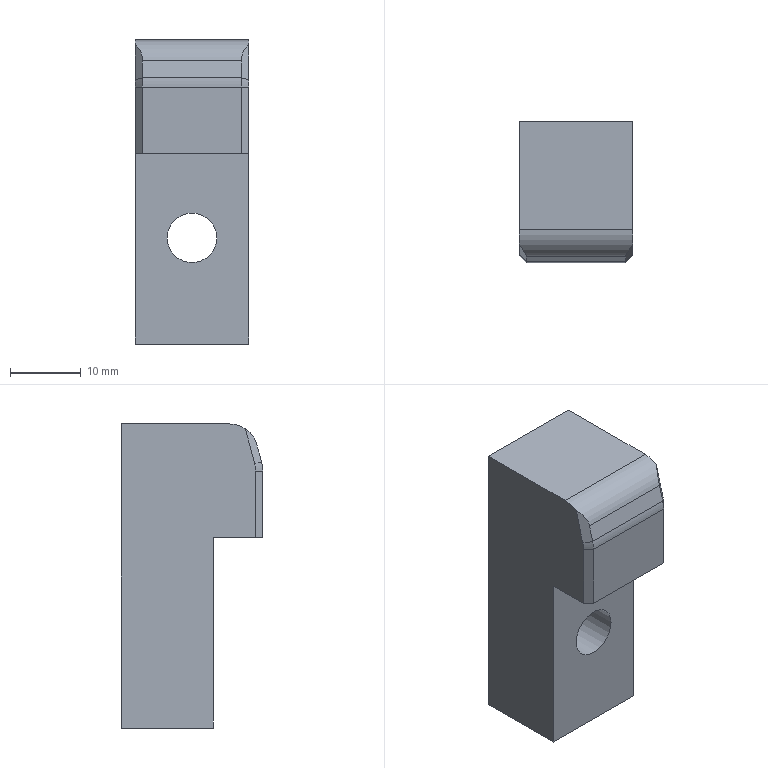Part | STEP file | gslz 2016.10.28-6_id702_x_t | 1 solid | 20 faces | box 16 x 20 x 42.992 mm | volume 9660 mm3 | plane 14 | cylinder 4 | cone 2 | commonest cylinder face diameters 7 x1 8 x1 10 x1 11 x1
STEP:
#1=CARTESIAN_POINT('',(115.2,205.01,79.));
#2=VERTEX_POINT('',#1);
#3=CARTESIAN_POINT('',(115.2,205.01,52.));
#4=VERTEX_POINT('',#3);
#5=CARTESIAN_POINT('',(115.2,205.01,69.));
#6=DIRECTION('',(0.000000258,0.,-1.));
#7=VECTOR('',#6,1.);
#8=LINE('',#5,#7);
#9=EDGE_CURVE('',#2,#4,#8,.T.);
#10=ORIENTED_EDGE('',*,*,#9,.F.);
#11=CARTESIAN_POINT('',(99.2,205.01,79.));
#12=VERTEX_POINT('',#11);
#13=CARTESIAN_POINT('',(100.2,205.01,79.));
#14=DIRECTION('',(1.,-0.000000182,0.000000244));
#15=VECTOR('',#14,1.);
#16=LINE('',#13,#15);
#17=EDGE_CURVE('',#12,#2,#16,.T.);
#18=ORIENTED_EDGE('',*,*,#17,.F.);
#19=CARTESIAN_POINT('',(99.2,205.01,52.));
#20=VERTEX_POINT('',#19);
#21=CARTESIAN_POINT('',(99.2,205.01,69.));
#22=DIRECTION('',(0.000000258,0.,-1.));
#23=VECTOR('',#22,1.);
#24=LINE('',#21,#23);
#25=EDGE_CURVE('',#12,#20,#24,.T.);
#26=ORIENTED_EDGE('',*,*,#25,.T.);
#27=CARTESIAN_POINT('',(43.45,205.01,52.));
#28=DIRECTION('',(1.,-0.000000182,0.));
#29=VECTOR('',#28,1.);
#30=LINE('',#27,#29);
#31=EDGE_CURVE('',#20,#4,#30,.T.);
#32=ORIENTED_EDGE('',*,*,#31,.T.);
#33=EDGE_LOOP('',(#10,#18,#26,#32));
#34=FACE_BOUND('',#33,.T.);
#35=CARTESIAN_POINT('',(110.7,205.01,67.));
#36=VERTEX_POINT('',#35);
#37=CARTESIAN_POINT('',(107.2,205.01,67.));
#38=DIRECTION('',(-0.000000182,-1.,0.));
#39=DIRECTION('',(1.,-0.000000182,0.000000244));
#40=AXIS2_PLACEMENT_3D('',#37,#38,#39);
#41=CIRCLE('',#40,3.5);
#42=EDGE_CURVE('',#36,#36,#41,.T.);
#43=ORIENTED_EDGE('',*,*,#42,.F.);
#44=EDGE_LOOP('',(#43));
#45=FACE_BOUND('',#44,.T.);
#46=CARTESIAN_POINT('',(100.2,205.01,79.));
#47=DIRECTION('',(-0.000000182,-1.,0.));
#48=DIRECTION('',(0.000000244,0.,-1.));
#49=AXIS2_PLACEMENT_3D('',#46,#47,#48);
#50=PLANE('',#49);
#51=ADVANCED_FACE('',(#34,#45),#50,.T.);
#52=CARTESIAN_POINT('',(114.2,198.01,79.));
#53=VERTEX_POINT('',#52);
#54=CARTESIAN_POINT('',(100.2,198.01,79.));
#55=VERTEX_POINT('',#54);
#56=CARTESIAN_POINT('',(338.566,198.01,79.));
#57=DIRECTION('',(-1.,0.000000182,-0.000000244));
#58=VECTOR('',#57,1.);
#59=LINE('',#56,#58);
#60=EDGE_CURVE('',#53,#55,#59,.T.);
#61=ORIENTED_EDGE('',*,*,#60,.F.);
#62=CARTESIAN_POINT('',(114.2,198.01,88.342));
#63=VERTEX_POINT('',#62);
#64=CARTESIAN_POINT('',(114.2,198.01,86.475));
#65=DIRECTION('',(-0.000000258,-0.000000001,1.));
#66=VECTOR('',#65,1.);
#67=LINE('',#64,#66);
#68=EDGE_CURVE('',#53,#63,#67,.T.);
#69=ORIENTED_EDGE('',*,*,#68,.T.);
#70=CARTESIAN_POINT('',(100.2,198.01,88.342));
#71=VERTEX_POINT('',#70);
#72=CARTESIAN_POINT('',(338.566,198.01,88.342));
#73=DIRECTION('',(-1.,0.000000182,-0.000000258));
#74=VECTOR('',#73,1.);
#75=LINE('',#72,#74);
#76=EDGE_CURVE('',#63,#71,#75,.T.);
#77=ORIENTED_EDGE('',*,*,#76,.T.);
#78=CARTESIAN_POINT('',(100.2,198.01,69.));
#79=DIRECTION('',(0.000000258,0.000000001,-1.));
#80=VECTOR('',#79,1.);
#81=LINE('',#78,#80);
#82=EDGE_CURVE('',#71,#55,#81,.T.);
#83=ORIENTED_EDGE('',*,*,#82,.T.);
#84=EDGE_LOOP('',(#61,#69,#77,#83));
#85=FACE_OUTER_BOUND('',#84,.T.);
#86=CARTESIAN_POINT('',(338.566,198.01,86.475));
#87=DIRECTION('',(-0.000000182,-1.,-0.000000001));
#88=DIRECTION('',(0.9986,-0.000000182,0.05234));
#89=AXIS2_PLACEMENT_3D('',#86,#87,#88);
#90=PLANE('',#89);
#91=ADVANCED_FACE('',(#85),#90,.T.);
#92=CARTESIAN_POINT('',(115.2,200.472,94.325));
#93=VERTEX_POINT('',#92);
#94=CARTESIAN_POINT('',(115.2,199.146,89.377));
#95=VERTEX_POINT('',#94);
#96=CARTESIAN_POINT('',(115.2,194.274,71.195));
#97=DIRECTION('',(0.000000152,-0.2588,-0.9659));
#98=VECTOR('',#97,1.);
#99=LINE('',#96,#98);
#100=EDGE_CURVE('',#93,#95,#99,.T.);
#101=ORIENTED_EDGE('',*,*,#100,.T.);
#102=CARTESIAN_POINT('',(115.2,199.01,88.342));
#103=VERTEX_POINT('',#102);
#104=CARTESIAN_POINT('',(115.2,203.01,88.342));
#105=DIRECTION('',(1.,-0.000000379,0.000000258));
#106=DIRECTION('',(0.000000379,1.,0.000000001));
#107=AXIS2_PLACEMENT_3D('',#104,#105,#106);
#108=CIRCLE('',#107,4.);
#109=EDGE_CURVE('',#95,#103,#108,.T.);
#110=ORIENTED_EDGE('',*,*,#109,.T.);
#111=CARTESIAN_POINT('',(115.2,199.01,79.));
#112=VERTEX_POINT('',#111);
#113=CARTESIAN_POINT('',(115.2,199.01,69.));
#114=DIRECTION('',(0.000000258,0.000000001,-1.));
#115=VECTOR('',#114,1.);
#116=LINE('',#113,#115);
#117=EDGE_CURVE('',#103,#112,#116,.T.);
#118=ORIENTED_EDGE('',*,*,#117,.T.);
#119=CARTESIAN_POINT('',(115.2,202.466,79.));
#120=DIRECTION('',(0.000000379,1.,0.));
#121=VECTOR('',#120,1.);
#122=LINE('',#119,#121);
#123=EDGE_CURVE('',#112,#2,#122,.T.);
#124=ORIENTED_EDGE('',*,*,#123,.T.);
#125=ORIENTED_EDGE('',*,*,#9,.T.);
#126=CARTESIAN_POINT('',(115.2,218.01,52.));
#127=VERTEX_POINT('',#126);
#128=CARTESIAN_POINT('',(115.2,-632.758,52.));
#129=DIRECTION('',(0.000000379,1.,0.));
#130=VECTOR('',#129,1.);
#131=LINE('',#128,#130);
#132=EDGE_CURVE('',#4,#127,#131,.T.);
#133=ORIENTED_EDGE('',*,*,#132,.T.);
#134=CARTESIAN_POINT('',(115.2,218.01,94.992));
#135=VERTEX_POINT('',#134);
#136=CARTESIAN_POINT('',(115.2,218.01,69.));
#137=DIRECTION('',(0.000000258,0.,-1.));
#138=VECTOR('',#137,1.);
#139=LINE('',#136,#138);
#140=EDGE_CURVE('',#135,#127,#139,.T.);
#141=ORIENTED_EDGE('',*,*,#140,.F.);
#142=CARTESIAN_POINT('',(115.2,202.685,94.992));
#143=VERTEX_POINT('',#142);
#144=CARTESIAN_POINT('',(115.2,150.,94.992));
#145=DIRECTION('',(0.000000379,1.,0.));
#146=VECTOR('',#145,1.);
#147=LINE('',#144,#146);
#148=EDGE_CURVE('',#143,#135,#147,.T.);
#149=ORIENTED_EDGE('',*,*,#148,.F.);
#150=CARTESIAN_POINT('',(115.2,202.685,90.992));
#151=DIRECTION('',(-1.,0.000000379,-0.000000258));
#152=DIRECTION('',(-0.000000379,-1.,0.));
#153=AXIS2_PLACEMENT_3D('',#150,#151,#152);
#154=CIRCLE('',#153,4.);
#155=EDGE_CURVE('',#93,#143,#154,.T.);
#156=ORIENTED_EDGE('',*,*,#155,.F.);
#157=EDGE_LOOP('',(#101,#110,#118,#124,#125,#133,#141,#149,#156));
#158=FACE_OUTER_BOUND('',#157,.T.);
#159=CARTESIAN_POINT('',(115.2,202.466,69.));
#160=DIRECTION('',(1.,-0.000000379,0.000000258));
#161=DIRECTION('',(-0.000000379,-1.,-0.000000001));
#162=AXIS2_PLACEMENT_3D('',#159,#160,#161);
#163=PLANE('',#162);
#164=ADVANCED_FACE('',(#158),#163,.T.);
#165=CARTESIAN_POINT('',(99.2,218.01,94.992));
#166=VERTEX_POINT('',#165);
#167=CARTESIAN_POINT('',(99.2,202.685,94.992));
#168=VERTEX_POINT('',#167);
#169=CARTESIAN_POINT('',(99.2,202.466,94.992));
#170=DIRECTION('',(-0.000000379,-1.,0.));
#171=VECTOR('',#170,1.);
#172=LINE('',#169,#171);
#173=EDGE_CURVE('',#166,#168,#172,.T.);
#174=ORIENTED_EDGE('',*,*,#173,.F.);
#175=CARTESIAN_POINT('',(99.2,218.01,52.));
#176=VERTEX_POINT('',#175);
#177=CARTESIAN_POINT('',(99.2,218.01,69.));
#178=DIRECTION('',(0.000000258,0.,-1.));
#179=VECTOR('',#178,1.);
#180=LINE('',#177,#179);
#181=EDGE_CURVE('',#166,#176,#180,.T.);
#182=ORIENTED_EDGE('',*,*,#181,.T.);
#183=CARTESIAN_POINT('',(99.2,-632.758,52.));
#184=DIRECTION('',(0.000000379,1.,0.));
#185=VECTOR('',#184,1.);
#186=LINE('',#183,#185);
#187=EDGE_CURVE('',#20,#176,#186,.T.);
#188=ORIENTED_EDGE('',*,*,#187,.F.);
#189=ORIENTED_EDGE('',*,*,#25,.F.);
#190=CARTESIAN_POINT('',(99.2,199.01,79.));
#191=VERTEX_POINT('',#190);
#192=CARTESIAN_POINT('',(99.2,202.466,79.));
#193=DIRECTION('',(-0.000000379,-1.,0.));
#194=VECTOR('',#193,1.);
#195=LINE('',#192,#194);
#196=EDGE_CURVE('',#12,#191,#195,.T.);
#197=ORIENTED_EDGE('',*,*,#196,.T.);
#198=CARTESIAN_POINT('',(99.2,199.01,88.342));
#199=VERTEX_POINT('',#198);
#200=CARTESIAN_POINT('',(99.2,199.01,88.342));
#201=DIRECTION('',(-0.000000258,-0.000000001,1.));
#202=VECTOR('',#201,1.);
#203=LINE('',#200,#202);
#204=EDGE_CURVE('',#191,#199,#203,.T.);
#205=ORIENTED_EDGE('',*,*,#204,.T.);
#206=CARTESIAN_POINT('',(99.2,199.146,89.377));
#207=VERTEX_POINT('',#206);
#208=CARTESIAN_POINT('',(99.2,203.01,88.342));
#209=DIRECTION('',(-1.,0.000000379,-0.000000258));
#210=DIRECTION('',(0.000000379,1.,0.000000001));
#211=AXIS2_PLACEMENT_3D('',#208,#209,#210);
#212=CIRCLE('',#211,4.);
#213=EDGE_CURVE('',#199,#207,#212,.T.);
#214=ORIENTED_EDGE('',*,*,#213,.T.);
#215=CARTESIAN_POINT('',(99.2,200.472,94.325));
#216=VERTEX_POINT('',#215);
#217=CARTESIAN_POINT('',(99.2,200.861,95.776));
#218=DIRECTION('',(-0.000000152,0.2588,0.9659));
#219=VECTOR('',#218,1.);
#220=LINE('',#217,#219);
#221=EDGE_CURVE('',#207,#216,#220,.T.);
#222=ORIENTED_EDGE('',*,*,#221,.T.);
#223=CARTESIAN_POINT('',(99.2,202.685,90.992));
#224=DIRECTION('',(1.,-0.000000379,0.000000258));
#225=DIRECTION('',(-0.000000379,-1.,0.));
#226=AXIS2_PLACEMENT_3D('',#223,#224,#225);
#227=CIRCLE('',#226,4.);
#228=EDGE_CURVE('',#168,#216,#227,.T.);
#229=ORIENTED_EDGE('',*,*,#228,.F.);
#230=EDGE_LOOP('',(#174,#182,#188,#189,#197,#205,#214,#222,#229));
#231=FACE_OUTER_BOUND('',#230,.T.);
#232=CARTESIAN_POINT('',(99.2,202.466,69.));
#233=DIRECTION('',(1.,-0.000000379,0.000000258));
#234=DIRECTION('',(-0.000000379,-1.,-0.000000001));
#235=AXIS2_PLACEMENT_3D('',#232,#233,#234);
#236=PLANE('',#235);
#237=ADVANCED_FACE('',(#231),#236,.F.);
#238=CARTESIAN_POINT('',(112.7,218.01,67.));
#239=VERTEX_POINT('',#238);
#240=CARTESIAN_POINT('',(107.2,218.01,67.));
#241=DIRECTION('',(-0.000000182,-1.,0.));
#242=DIRECTION('',(1.,-0.000000182,0.));
#243=AXIS2_PLACEMENT_3D('',#240,#241,#242);
#244=CIRCLE('',#243,5.5);
#245=EDGE_CURVE('',#239,#239,#244,.T.);
#246=ORIENTED_EDGE('',*,*,#245,.T.);
#247=EDGE_LOOP('',(#246));
#248=FACE_BOUND('',#247,.T.);
#249=ORIENTED_EDGE('',*,*,#140,.T.);
#250=CARTESIAN_POINT('',(43.45,218.01,52.));
#251=DIRECTION('',(1.,-0.000000182,0.));
#252=VECTOR('',#251,1.);
#253=LINE('',#250,#252);
#254=EDGE_CURVE('',#176,#127,#253,.T.);
#255=ORIENTED_EDGE('',*,*,#254,.F.);
#256=ORIENTED_EDGE('',*,*,#181,.F.);
#257=CARTESIAN_POINT('',(100.2,218.01,94.992));
#258=DIRECTION('',(-1.,0.000000182,0.));
#259=VECTOR('',#258,1.);
#260=LINE('',#257,#259);
#261=EDGE_CURVE('',#135,#166,#260,.T.);
#262=ORIENTED_EDGE('',*,*,#261,.F.);
#263=EDGE_LOOP('',(#249,#255,#256,#262));
#264=FACE_BOUND('',#263,.T.);
#265=CARTESIAN_POINT('',(100.2,218.01,79.));
#266=DIRECTION('',(-0.000000182,-1.,0.));
#267=DIRECTION('',(0.000000244,0.,-1.));
#268=AXIS2_PLACEMENT_3D('',#265,#266,#267);
#269=PLANE('',#268);
#270=ADVANCED_FACE('',(#248,#264),#269,.F.);
#271=CARTESIAN_POINT('',(100.2,198.18,89.636));
#272=VERTEX_POINT('',#271);
#273=CARTESIAN_POINT('',(114.2,198.18,89.636));
#274=VERTEX_POINT('',#273);
#275=CARTESIAN_POINT('',(113.7,198.18,89.636));
#276=DIRECTION('',(1.,-0.000000182,0.000000258));
#277=VECTOR('',#276,1.);
#278=LINE('',#275,#277);
#279=EDGE_CURVE('',#272,#274,#278,.T.);
#280=ORIENTED_EDGE('',*,*,#279,.T.);
#281=CARTESIAN_POINT('',(114.2,198.821,92.028));
#282=VERTEX_POINT('',#281);
#283=CARTESIAN_POINT('',(114.2,200.51,98.33));
#284=DIRECTION('',(-0.000000152,0.2588,0.9659));
#285=VECTOR('',#284,1.);
#286=LINE('',#283,#285);
#287=EDGE_CURVE('',#274,#282,#286,.T.);
#288=ORIENTED_EDGE('',*,*,#287,.T.);
#289=CARTESIAN_POINT('',(100.2,198.821,92.028));
#290=VERTEX_POINT('',#289);
#291=CARTESIAN_POINT('',(113.7,198.821,92.028));
#292=DIRECTION('',(-1.,0.000000252,0.));
#293=VECTOR('',#292,1.);
#294=LINE('',#291,#293);
#295=EDGE_CURVE('',#282,#290,#294,.T.);
#296=ORIENTED_EDGE('',*,*,#295,.T.);
#297=CARTESIAN_POINT('',(100.2,198.18,89.636));
#298=DIRECTION('',(0.000000152,-0.2588,-0.9659));
#299=VECTOR('',#298,1.);
#300=LINE('',#297,#299);
#301=EDGE_CURVE('',#290,#272,#300,.T.);
#302=ORIENTED_EDGE('',*,*,#301,.T.);
#303=EDGE_LOOP('',(#280,#288,#296,#302));
#304=FACE_OUTER_BOUND('',#303,.T.);
#305=CARTESIAN_POINT('',(113.7,200.51,98.33));
#306=DIRECTION('',(-0.000000243,-0.9659,0.2588));
#307=DIRECTION('',(-1.,0.000000182,-0.000000258));
#308=AXIS2_PLACEMENT_3D('',#305,#306,#307);
#309=PLANE('',#308);
#310=ADVANCED_FACE('',(#304),#309,.T.);
#311=ORIENTED_EDGE('',*,*,#148,.T.);
#312=ORIENTED_EDGE('',*,*,#261,.T.);
#313=ORIENTED_EDGE('',*,*,#173,.T.);
#314=CARTESIAN_POINT('',(-2.,202.685,94.992));
#315=DIRECTION('',(1.,-0.000000252,0.));
#316=VECTOR('',#315,1.);
#317=LINE('',#314,#316);
#318=EDGE_CURVE('',#168,#143,#317,.T.);
#319=ORIENTED_EDGE('',*,*,#318,.T.);
#320=EDGE_LOOP('',(#311,#312,#313,#319));
#321=FACE_OUTER_BOUND('',#320,.T.);
#322=CARTESIAN_POINT('',(-2.,150.,94.992));
#323=DIRECTION('',(0.,0.,1.));
#324=DIRECTION('',(1.,0.,0.));
#325=AXIS2_PLACEMENT_3D('',#322,#323,#324);
#326=PLANE('',#325);
#327=ADVANCED_FACE('',(#321),#326,.T.);
#328=ORIENTED_EDGE('',*,*,#228,.T.);
#329=CARTESIAN_POINT('',(96.2,202.685,90.992));
#330=DIRECTION('',(0.7071,0.683,-0.183));
#331=DIRECTION('',(0.7071,-0.683,0.183));
#332=AXIS2_PLACEMENT_3D('',#329,#330,#331);
#333=ELLIPSE('',#332,5.657,4.);
#334=EDGE_CURVE('',#216,#290,#333,.T.);
#335=ORIENTED_EDGE('',*,*,#334,.T.);
#336=ORIENTED_EDGE('',*,*,#295,.F.);
#337=CARTESIAN_POINT('',(118.2,202.685,90.992));
#338=DIRECTION('',(0.7071,-0.683,0.183));
#339=DIRECTION('',(0.7071,0.683,-0.183));
#340=AXIS2_PLACEMENT_3D('',#337,#338,#339);
#341=ELLIPSE('',#340,5.657,4.);
#342=EDGE_CURVE('',#93,#282,#341,.T.);
#343=ORIENTED_EDGE('',*,*,#342,.F.);
#344=ORIENTED_EDGE('',*,*,#155,.T.);
#345=ORIENTED_EDGE('',*,*,#318,.F.);
#346=EDGE_LOOP('',(#328,#335,#336,#343,#344,#345));
#347=FACE_OUTER_BOUND('',#346,.T.);
#348=CARTESIAN_POINT('',(113.7,202.685,90.992));
#349=DIRECTION('',(1.,-0.000000252,0.));
#350=DIRECTION('',(0.000000252,1.,0.));
#351=AXIS2_PLACEMENT_3D('',#348,#349,#350);
#352=CYLINDRICAL_SURFACE('',#351,4.);
#353=ADVANCED_FACE('',(#347),#352,.T.);
#354=ORIENTED_EDGE('',*,*,#76,.F.);
#355=CARTESIAN_POINT('',(114.2,203.01,88.342));
#356=DIRECTION('',(-1.,0.000000182,-0.000000258));
#357=DIRECTION('',(0.000000182,1.,0.000000001));
#358=AXIS2_PLACEMENT_3D('',#355,#356,#357);
#359=CIRCLE('',#358,5.);
#360=EDGE_CURVE('',#63,#274,#359,.T.);
#361=ORIENTED_EDGE('',*,*,#360,.T.);
#362=ORIENTED_EDGE('',*,*,#279,.F.);
#363=CARTESIAN_POINT('',(100.2,203.01,88.342));
#364=DIRECTION('',(1.,-0.000000182,0.000000258));
#365=DIRECTION('',(0.000000182,1.,0.000000001));
#366=AXIS2_PLACEMENT_3D('',#363,#364,#365);
#367=CIRCLE('',#366,5.);
#368=EDGE_CURVE('',#272,#71,#367,.T.);
#369=ORIENTED_EDGE('',*,*,#368,.T.);
#370=EDGE_LOOP('',(#354,#361,#362,#369));
#371=FACE_OUTER_BOUND('',#370,.T.);
#372=CARTESIAN_POINT('',(338.566,203.01,88.342));
#373=DIRECTION('',(-1.,0.000000182,-0.000000258));
#374=DIRECTION('',(-0.000000258,0.,1.));
#375=AXIS2_PLACEMENT_3D('',#372,#373,#374);
#376=CYLINDRICAL_SURFACE('',#375,5.);
#377=ADVANCED_FACE('',(#371),#376,.T.);
#378=CARTESIAN_POINT('',(114.2,198.01,79.));
#379=DIRECTION('',(-0.7071,-0.7071,-0.000000172));
#380=VECTOR('',#379,1.);
#381=LINE('',#378,#380);
#382=EDGE_CURVE('',#112,#53,#381,.T.);
#383=ORIENTED_EDGE('',*,*,#382,.F.);
#384=ORIENTED_EDGE('',*,*,#117,.F.);
#385=CARTESIAN_POINT('',(114.2,198.01,88.342));
#386=DIRECTION('',(0.7071,0.7071,0.000000184));
#387=VECTOR('',#386,1.);
#388=LINE('',#385,#387);
#389=EDGE_CURVE('',#63,#103,#388,.T.);
#390=ORIENTED_EDGE('',*,*,#389,.F.);
#391=ORIENTED_EDGE('',*,*,#68,.F.);
#392=EDGE_LOOP('',(#383,#384,#390,#391));
#393=FACE_OUTER_BOUND('',#392,.T.);
#394=CARTESIAN_POINT('',(114.2,198.01,86.475));
#395=DIRECTION('',(-0.7071,0.7071,-0.000000182));
#396=DIRECTION('',(0.000000258,0.000000001,-1.));
#397=AXIS2_PLACEMENT_3D('',#394,#395,#396);
#398=PLANE('',#397);
#399=ADVANCED_FACE('',(#393),#398,.F.);
#400=ORIENTED_EDGE('',*,*,#389,.T.);
#401=ORIENTED_EDGE('',*,*,#109,.F.);
#402=CARTESIAN_POINT('',(114.2,198.18,89.636));
#403=DIRECTION('',(0.7071,0.683,-0.183));
#404=VECTOR('',#403,1.);
#405=LINE('',#402,#404);
#406=EDGE_CURVE('',#274,#95,#405,.T.);
#407=ORIENTED_EDGE('',*,*,#406,.F.);
#408=ORIENTED_EDGE('',*,*,#360,.F.);
#409=EDGE_LOOP('',(#400,#401,#407,#408));
#410=FACE_OUTER_BOUND('',#409,.T.);
#411=CARTESIAN_POINT('',(115.2,203.01,88.342));
#412=DIRECTION('',(-1.,0.000000182,-0.000000258));
#413=DIRECTION('',(-0.000000182,-1.,-0.000000001));
#414=AXIS2_PLACEMENT_3D('',#411,#412,#413);
#415=CONICAL_SURFACE('',#414,4.,45.);
#416=ADVANCED_FACE('',(#410),#415,.T.);
#417=ORIENTED_EDGE('',*,*,#406,.T.);
#418=ORIENTED_EDGE('',*,*,#100,.F.);
#419=ORIENTED_EDGE('',*,*,#342,.T.);
#420=ORIENTED_EDGE('',*,*,#287,.F.);
#421=EDGE_LOOP('',(#417,#418,#419,#420));
#422=FACE_OUTER_BOUND('',#421,.T.);
#423=CARTESIAN_POINT('',(115.2,194.274,71.195));
#424=DIRECTION('',(-0.7071,0.683,-0.183));
#425=DIRECTION('',(-0.000000152,0.2588,0.9659));
#426=AXIS2_PLACEMENT_3D('',#423,#424,#425);
#427=PLANE('',#426);
#428=ADVANCED_FACE('',(#422),#427,.F.);
#429=ORIENTED_EDGE('',*,*,#221,.F.);
#430=CARTESIAN_POINT('',(99.7,198.663,89.506));
#431=DIRECTION('',(-0.7071,0.683,-0.183));
#432=VECTOR('',#431,1.);
#433=LINE('',#430,#432);
#434=EDGE_CURVE('',#272,#207,#433,.T.);
#435=ORIENTED_EDGE('',*,*,#434,.F.);
#436=ORIENTED_EDGE('',*,*,#301,.F.);
#437=ORIENTED_EDGE('',*,*,#334,.F.);
#438=EDGE_LOOP('',(#429,#435,#436,#437));
#439=FACE_OUTER_BOUND('',#438,.T.);
#440=CARTESIAN_POINT('',(100.2,200.51,98.33));
#441=DIRECTION('',(-0.7071,-0.683,0.183));
#442=DIRECTION('',(0.6947,-0.7193,0.));
#443=AXIS2_PLACEMENT_3D('',#440,#441,#442);
#444=PLANE('',#443);
#445=ADVANCED_FACE('',(#439),#444,.T.);
#446=ORIENTED_EDGE('',*,*,#434,.T.);
#447=ORIENTED_EDGE('',*,*,#213,.F.);
#448=CARTESIAN_POINT('',(99.7,198.51,88.342));
#449=DIRECTION('',(-0.7071,0.7071,-0.000000084));
#450=VECTOR('',#449,1.);
#451=LINE('',#448,#450);
#452=EDGE_CURVE('',#71,#199,#451,.T.);
#453=ORIENTED_EDGE('',*,*,#452,.F.);
#454=ORIENTED_EDGE('',*,*,#368,.F.);
#455=EDGE_LOOP('',(#446,#447,#453,#454));
#456=FACE_OUTER_BOUND('',#455,.T.);
#457=CARTESIAN_POINT('',(99.2,203.01,88.342));
#458=DIRECTION('',(1.,-0.000000182,0.000000258));
#459=DIRECTION('',(0.000000182,1.,0.000000001));
#460=AXIS2_PLACEMENT_3D('',#457,#458,#459);
#461=CONICAL_SURFACE('',#460,4.,45.);
#462=ADVANCED_FACE('',(#456),#461,.T.);
#463=CARTESIAN_POINT('',(99.2,199.01,79.));
#464=DIRECTION('',(-0.7071,0.7071,-0.000000172));
#465=VECTOR('',#464,1.);
#466=LINE('',#463,#465);
#467=EDGE_CURVE('',#55,#191,#466,.T.);
#468=ORIENTED_EDGE('',*,*,#467,.F.);
#469=ORIENTED_EDGE('',*,*,#82,.F.);
#470=ORIENTED_EDGE('',*,*,#452,.T.);
#471=ORIENTED_EDGE('',*,*,#204,.F.);
#472=EDGE_LOOP('',(#468,#469,#470,#471));
#473=FACE_OUTER_BOUND('',#472,.T.);
#474=CARTESIAN_POINT('',(99.2,199.01,69.));
#475=DIRECTION('',(-0.7071,-0.7071,-0.000000184));
#476=DIRECTION('',(-0.000000258,-0.000000001,1.));
#477=AXIS2_PLACEMENT_3D('',#474,#475,#476);
#478=PLANE('',#477);
#479=ADVANCED_FACE('',(#473),#478,.T.);
#480=ORIENTED_EDGE('',*,*,#196,.F.);
#481=ORIENTED_EDGE('',*,*,#17,.T.);
#482=ORIENTED_EDGE('',*,*,#123,.F.);
#483=ORIENTED_EDGE('',*,*,#382,.T.);
#484=ORIENTED_EDGE('',*,*,#60,.T.);
#485=ORIENTED_EDGE('',*,*,#467,.T.);
#486=EDGE_LOOP('',(#480,#481,#482,#483,#484,#485));
#487=FACE_OUTER_BOUND('',#486,.T.);
#488=CARTESIAN_POINT('',(107.7,212.184,79.));
#489=DIRECTION('',(-0.000000244,0.,1.));
#490=DIRECTION('',(1.,-0.000000182,0.000000244));
#491=AXIS2_PLACEMENT_3D('',#488,#489,#490);
#492=PLANE('',#491);
#493=ADVANCED_FACE('',(#487),#492,.F.);
#494=ORIENTED_EDGE('',*,*,#31,.F.);
#495=ORIENTED_EDGE('',*,*,#187,.T.);
#496=ORIENTED_EDGE('',*,*,#254,.T.);
#497=ORIENTED_EDGE('',*,*,#132,.F.);
#498=EDGE_LOOP('',(#494,#495,#496,#497));
#499=FACE_OUTER_BOUND('',#498,.T.);
#500=CARTESIAN_POINT('',(43.45,-632.758,52.));
#501=DIRECTION('',(0.,0.,1.));
#502=DIRECTION('',(0.,-1.,0.));
#503=AXIS2_PLACEMENT_3D('',#500,#501,#502);
#504=PLANE('',#503);
#505=ADVANCED_FACE('',(#499),#504,.F.);
#506=ORIENTED_EDGE('',*,*,#42,.T.);
#507=EDGE_LOOP('',(#506));
#508=FACE_BOUND('',#507,.T.);
#509=CARTESIAN_POINT('',(110.7,210.01,67.));
#510=VERTEX_POINT('',#509);
#511=CARTESIAN_POINT('',(107.2,210.01,67.));
#512=DIRECTION('',(0.000000182,1.,0.));
#513=DIRECTION('',(1.,-0.000000182,0.000000244));
#514=AXIS2_PLACEMENT_3D('',#511,#512,#513);
#515=CIRCLE('',#514,3.5);
#516=EDGE_CURVE('',#510,#510,#515,.T.);
#517=ORIENTED_EDGE('',*,*,#516,.T.);
#518=EDGE_LOOP('',(#517));
#519=FACE_BOUND('',#518,.T.);
#520=CARTESIAN_POINT('',(107.2,204.184,67.));
#521=DIRECTION('',(-0.000000182,-1.,0.));
#522=DIRECTION('',(1.,-0.000000182,0.));
#523=AXIS2_PLACEMENT_3D('',#520,#521,#522);
#524=CYLINDRICAL_SURFACE('',#523,3.5);
#525=ADVANCED_FACE('',(#508,#519),#524,.F.);
#526=ORIENTED_EDGE('',*,*,#516,.F.);
#527=EDGE_LOOP('',(#526));
#528=FACE_BOUND('',#527,.T.);
#529=CARTESIAN_POINT('',(112.7,210.01,67.));
#530=VERTEX_POINT('',#529);
#531=CARTESIAN_POINT('',(107.2,210.01,67.));
#532=DIRECTION('',(0.000000182,1.,0.));
#533=DIRECTION('',(1.,-0.000000182,0.000000244));
#534=AXIS2_PLACEMENT_3D('',#531,#532,#533);
#535=CIRCLE('',#534,5.5);
#536=EDGE_CURVE('',#530,#530,#535,.T.);
#537=ORIENTED_EDGE('',*,*,#536,.T.);
#538=EDGE_LOOP('',(#537));
#539=FACE_BOUND('',#538,.T.);
#540=CARTESIAN_POINT('',(107.2,210.01,67.));
#541=DIRECTION('',(-0.000000182,-1.,0.));
#542=DIRECTION('',(-1.,0.000000182,-0.000000244));
#543=AXIS2_PLACEMENT_3D('',#540,#541,#542);
#544=PLANE('',#543);
#545=ADVANCED_FACE('',(#528,#539),#544,.F.);
#546=ORIENTED_EDGE('',*,*,#245,.F.);
#547=EDGE_LOOP('',(#546));
#548=FACE_BOUND('',#547,.T.);
#549=ORIENTED_EDGE('',*,*,#536,.F.);
#550=EDGE_LOOP('',(#549));
#551=FACE_BOUND('',#550,.T.);
#552=CARTESIAN_POINT('',(107.2,219.184,67.));
#553=DIRECTION('',(-0.000000182,-1.,0.));
#554=DIRECTION('',(1.,-0.000000182,0.));
#555=AXIS2_PLACEMENT_3D('',#552,#553,#554);
#556=CYLINDRICAL_SURFACE('',#555,5.5);
#557=ADVANCED_FACE('',(#548,#551),#556,.F.);
#558=CLOSED_SHELL('',(#51,#91,#164,#237,#270,#310,#327,#353,#377,#399,#416,#428,#445,#462,#479,#493,#505,#525,#545,#557));
#559=MANIFOLD_SOLID_BREP('',#558);
#560=(LENGTH_UNIT()NAMED_UNIT(*)SI_UNIT(.MILLI.,.METRE.));
#561=UNCERTAINTY_MEASURE_WITH_UNIT(LENGTH_MEASURE(0.00002),#560,'','');
#562=(NAMED_UNIT(*)PLANE_ANGLE_UNIT()SI_UNIT($,.RADIAN.));
#563=PLANE_ANGLE_MEASURE_WITH_UNIT(PLANE_ANGLE_MEASURE(0.01745),#562);
#564=DIMENSIONAL_EXPONENTS(0.,0.,0.,0.,0.,0.,0.);
#565=(CONVERSION_BASED_UNIT('DEGREE',#563)NAMED_UNIT(#564)PLANE_ANGLE_UNIT());
#566=(NAMED_UNIT(*)SI_UNIT($,.STERADIAN.)SOLID_ANGLE_UNIT());
#567=(GEOMETRIC_REPRESENTATION_CONTEXT(3)GLOBAL_UNCERTAINTY_ASSIGNED_CONTEXT((#561))GLOBAL_UNIT_ASSIGNED_CONTEXT((#560,#565,#566))REPRESENTATION_CONTEXT('',''));
#568=ADVANCED_BREP_SHAPE_REPRESENTATION('',(#559),#567);